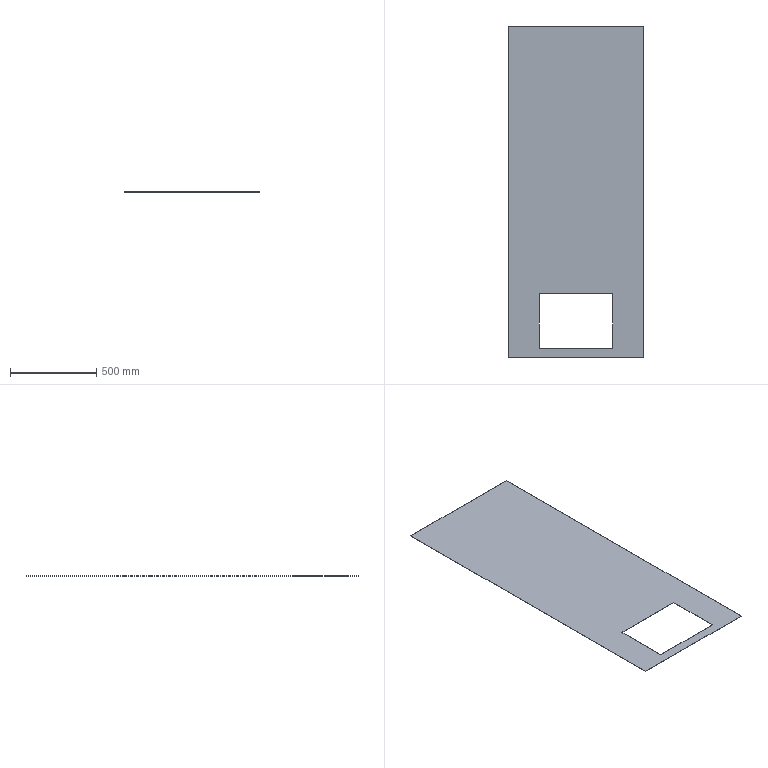Part | STEP file | 750078414 | 1 solid | 10 faces | box 785 x 1925 x 1.5 mm | volume 2064757 mm3 | plane 10
STEP:
#1=CARTESIAN_POINT('',(212.,-589.,1.5));
#2=VERTEX_POINT('',#1);
#3=CARTESIAN_POINT('',(212.,-906.5,1.5));
#4=VERTEX_POINT('',#3);
#5=CARTESIAN_POINT('',(212.,0.,1.5));
#6=DIRECTION('',(0.,-1.,0.));
#7=VECTOR('',#6,1000.);
#8=LINE('',#5,#7);
#9=EDGE_CURVE('',#2,#4,#8,.T.);
#10=ORIENTED_EDGE('',*,*,#9,.T.);
#11=CARTESIAN_POINT('',(-212.,-906.5,1.5));
#12=VERTEX_POINT('',#11);
#13=CARTESIAN_POINT('',(0.,-906.5,1.5));
#14=DIRECTION('',(-1.,0.,0.));
#15=VECTOR('',#14,1000.);
#16=LINE('',#13,#15);
#17=EDGE_CURVE('',#4,#12,#16,.T.);
#18=ORIENTED_EDGE('',*,*,#17,.T.);
#19=CARTESIAN_POINT('',(-212.,-589.,1.5));
#20=VERTEX_POINT('',#19);
#21=CARTESIAN_POINT('',(-212.,0.,1.5));
#22=DIRECTION('',(0.,1.,0.));
#23=VECTOR('',#22,1000.);
#24=LINE('',#21,#23);
#25=EDGE_CURVE('',#12,#20,#24,.T.);
#26=ORIENTED_EDGE('',*,*,#25,.T.);
#27=CARTESIAN_POINT('',(0.,-589.,1.5));
#28=DIRECTION('',(1.,0.,0.));
#29=VECTOR('',#28,1000.);
#30=LINE('',#27,#29);
#31=EDGE_CURVE('',#20,#2,#30,.T.);
#32=ORIENTED_EDGE('',*,*,#31,.T.);
#33=EDGE_LOOP('',(#10,#18,#26,#32));
#34=FACE_BOUND('',#33,.T.);
#35=CARTESIAN_POINT('',(-392.5,-962.5,1.5));
#36=VERTEX_POINT('',#35);
#37=CARTESIAN_POINT('',(392.5,-962.5,1.5));
#38=VERTEX_POINT('',#37);
#39=CARTESIAN_POINT('',(0.,-962.5,1.5));
#40=DIRECTION('',(1.,0.,0.));
#41=VECTOR('',#40,1000.);
#42=LINE('',#39,#41);
#43=EDGE_CURVE('',#36,#38,#42,.T.);
#44=ORIENTED_EDGE('',*,*,#43,.T.);
#45=CARTESIAN_POINT('',(392.5,962.5,1.5));
#46=VERTEX_POINT('',#45);
#47=CARTESIAN_POINT('',(392.5,0.,1.5));
#48=DIRECTION('',(0.,1.,0.));
#49=VECTOR('',#48,1000.);
#50=LINE('',#47,#49);
#51=EDGE_CURVE('',#38,#46,#50,.T.);
#52=ORIENTED_EDGE('',*,*,#51,.T.);
#53=CARTESIAN_POINT('',(-392.5,962.5,1.5));
#54=VERTEX_POINT('',#53);
#55=CARTESIAN_POINT('',(0.,962.5,1.5));
#56=DIRECTION('',(-1.,0.,0.));
#57=VECTOR('',#56,1000.);
#58=LINE('',#55,#57);
#59=EDGE_CURVE('',#46,#54,#58,.T.);
#60=ORIENTED_EDGE('',*,*,#59,.T.);
#61=CARTESIAN_POINT('',(-392.5,0.,1.5));
#62=DIRECTION('',(0.,-1.,0.));
#63=VECTOR('',#62,1000.);
#64=LINE('',#61,#63);
#65=EDGE_CURVE('',#54,#36,#64,.T.);
#66=ORIENTED_EDGE('',*,*,#65,.T.);
#67=EDGE_LOOP('',(#44,#52,#60,#66));
#68=FACE_OUTER_BOUND('',#67,.T.);
#69=CARTESIAN_POINT('',(0.,0.,1.5));
#70=DIRECTION('',(0.,0.,1.));
#71=DIRECTION('',(1.,0.,0.));
#72=AXIS2_PLACEMENT_3D('',#69,#70,#71);
#73=PLANE('',#72);
#74=ADVANCED_FACE('',(#34,#68),#73,.T.);
#75=CARTESIAN_POINT('',(-212.,-906.5,0.));
#76=VERTEX_POINT('',#75);
#77=CARTESIAN_POINT('',(-212.,-906.5,2078.907));
#78=DIRECTION('',(0.,0.,1.));
#79=VECTOR('',#78,1000.);
#80=LINE('',#77,#79);
#81=EDGE_CURVE('',#76,#12,#80,.T.);
#82=ORIENTED_EDGE('',*,*,#81,.T.);
#83=ORIENTED_EDGE('',*,*,#17,.F.);
#84=CARTESIAN_POINT('',(212.,-906.5,0.));
#85=VERTEX_POINT('',#84);
#86=CARTESIAN_POINT('',(212.,-906.5,2078.907));
#87=DIRECTION('',(0.,0.,-1.));
#88=VECTOR('',#87,1000.);
#89=LINE('',#86,#88);
#90=EDGE_CURVE('',#4,#85,#89,.T.);
#91=ORIENTED_EDGE('',*,*,#90,.T.);
#92=CARTESIAN_POINT('',(-212.,-906.5,0.));
#93=DIRECTION('',(-1.,0.,0.));
#94=VECTOR('',#93,1000.);
#95=LINE('',#92,#94);
#96=EDGE_CURVE('',#85,#76,#95,.T.);
#97=ORIENTED_EDGE('',*,*,#96,.T.);
#98=EDGE_LOOP('',(#82,#83,#91,#97));
#99=FACE_OUTER_BOUND('',#98,.T.);
#100=CARTESIAN_POINT('',(-212.,-906.5,2078.907));
#101=DIRECTION('',(0.,1.,0.));
#102=DIRECTION('',(0.,0.,1.));
#103=AXIS2_PLACEMENT_3D('',#100,#101,#102);
#104=PLANE('',#103);
#105=ADVANCED_FACE('',(#99),#104,.T.);
#106=ORIENTED_EDGE('',*,*,#90,.F.);
#107=ORIENTED_EDGE('',*,*,#9,.F.);
#108=CARTESIAN_POINT('',(212.,-589.,0.));
#109=VERTEX_POINT('',#108);
#110=CARTESIAN_POINT('',(212.,-589.,2078.907));
#111=DIRECTION('',(0.,0.,-1.));
#112=VECTOR('',#111,1000.);
#113=LINE('',#110,#112);
#114=EDGE_CURVE('',#2,#109,#113,.T.);
#115=ORIENTED_EDGE('',*,*,#114,.T.);
#116=CARTESIAN_POINT('',(212.,-906.5,0.));
#117=DIRECTION('',(0.,-1.,0.));
#118=VECTOR('',#117,1000.);
#119=LINE('',#116,#118);
#120=EDGE_CURVE('',#109,#85,#119,.T.);
#121=ORIENTED_EDGE('',*,*,#120,.T.);
#122=EDGE_LOOP('',(#106,#107,#115,#121));
#123=FACE_OUTER_BOUND('',#122,.T.);
#124=CARTESIAN_POINT('',(212.,-906.5,2078.907));
#125=DIRECTION('',(-1.,0.,0.));
#126=DIRECTION('',(0.,-1.,0.));
#127=AXIS2_PLACEMENT_3D('',#124,#125,#126);
#128=PLANE('',#127);
#129=ADVANCED_FACE('',(#123),#128,.T.);
#130=ORIENTED_EDGE('',*,*,#114,.F.);
#131=ORIENTED_EDGE('',*,*,#31,.F.);
#132=CARTESIAN_POINT('',(-212.,-589.,0.));
#133=VERTEX_POINT('',#132);
#134=CARTESIAN_POINT('',(-212.,-589.,2078.907));
#135=DIRECTION('',(0.,0.,-1.));
#136=VECTOR('',#135,1000.);
#137=LINE('',#134,#136);
#138=EDGE_CURVE('',#20,#133,#137,.T.);
#139=ORIENTED_EDGE('',*,*,#138,.T.);
#140=CARTESIAN_POINT('',(212.,-589.,0.));
#141=DIRECTION('',(1.,0.,0.));
#142=VECTOR('',#141,1000.);
#143=LINE('',#140,#142);
#144=EDGE_CURVE('',#133,#109,#143,.T.);
#145=ORIENTED_EDGE('',*,*,#144,.T.);
#146=EDGE_LOOP('',(#130,#131,#139,#145));
#147=FACE_OUTER_BOUND('',#146,.T.);
#148=CARTESIAN_POINT('',(212.,-589.,2078.907));
#149=DIRECTION('',(0.,-1.,0.));
#150=DIRECTION('',(0.,0.,-1.));
#151=AXIS2_PLACEMENT_3D('',#148,#149,#150);
#152=PLANE('',#151);
#153=ADVANCED_FACE('',(#147),#152,.T.);
#154=ORIENTED_EDGE('',*,*,#138,.F.);
#155=ORIENTED_EDGE('',*,*,#25,.F.);
#156=ORIENTED_EDGE('',*,*,#81,.F.);
#157=CARTESIAN_POINT('',(-212.,-589.,0.));
#158=DIRECTION('',(0.,1.,0.));
#159=VECTOR('',#158,1000.);
#160=LINE('',#157,#159);
#161=EDGE_CURVE('',#76,#133,#160,.T.);
#162=ORIENTED_EDGE('',*,*,#161,.T.);
#163=EDGE_LOOP('',(#154,#155,#156,#162));
#164=FACE_OUTER_BOUND('',#163,.T.);
#165=CARTESIAN_POINT('',(-212.,-589.,2078.907));
#166=DIRECTION('',(1.,0.,0.));
#167=DIRECTION('',(0.,1.,0.));
#168=AXIS2_PLACEMENT_3D('',#165,#166,#167);
#169=PLANE('',#168);
#170=ADVANCED_FACE('',(#164),#169,.T.);
#171=CARTESIAN_POINT('',(392.5,962.5,0.));
#172=VERTEX_POINT('',#171);
#173=CARTESIAN_POINT('',(392.5,962.5,1.5));
#174=DIRECTION('',(0.,0.,-1.));
#175=VECTOR('',#174,1000.);
#176=LINE('',#173,#175);
#177=EDGE_CURVE('',#46,#172,#176,.T.);
#178=ORIENTED_EDGE('',*,*,#177,.F.);
#179=ORIENTED_EDGE('',*,*,#51,.F.);
#180=CARTESIAN_POINT('',(392.5,-962.5,0.));
#181=VERTEX_POINT('',#180);
#182=CARTESIAN_POINT('',(392.5,-962.5,1.5));
#183=DIRECTION('',(0.,0.,1.));
#184=VECTOR('',#183,1000.);
#185=LINE('',#182,#184);
#186=EDGE_CURVE('',#181,#38,#185,.T.);
#187=ORIENTED_EDGE('',*,*,#186,.F.);
#188=CARTESIAN_POINT('',(392.5,-962.5,0.));
#189=DIRECTION('',(0.,-1.,0.));
#190=VECTOR('',#189,1000.);
#191=LINE('',#188,#190);
#192=EDGE_CURVE('',#172,#181,#191,.T.);
#193=ORIENTED_EDGE('',*,*,#192,.F.);
#194=EDGE_LOOP('',(#178,#179,#187,#193));
#195=FACE_OUTER_BOUND('',#194,.T.);
#196=CARTESIAN_POINT('',(392.5,-962.5,1.5));
#197=DIRECTION('',(-1.,0.,0.));
#198=DIRECTION('',(0.,0.,1.));
#199=AXIS2_PLACEMENT_3D('',#196,#197,#198);
#200=PLANE('',#199);
#201=ADVANCED_FACE('',(#195),#200,.F.);
#202=ORIENTED_EDGE('',*,*,#186,.T.);
#203=ORIENTED_EDGE('',*,*,#43,.F.);
#204=CARTESIAN_POINT('',(-392.5,-962.5,0.));
#205=VERTEX_POINT('',#204);
#206=CARTESIAN_POINT('',(-392.5,-962.5,1.5));
#207=DIRECTION('',(0.,0.,1.));
#208=VECTOR('',#207,1000.);
#209=LINE('',#206,#208);
#210=EDGE_CURVE('',#205,#36,#209,.T.);
#211=ORIENTED_EDGE('',*,*,#210,.F.);
#212=CARTESIAN_POINT('',(-392.5,-962.5,0.));
#213=DIRECTION('',(-1.,0.,0.));
#214=VECTOR('',#213,1000.);
#215=LINE('',#212,#214);
#216=EDGE_CURVE('',#181,#205,#215,.T.);
#217=ORIENTED_EDGE('',*,*,#216,.F.);
#218=EDGE_LOOP('',(#202,#203,#211,#217));
#219=FACE_OUTER_BOUND('',#218,.T.);
#220=CARTESIAN_POINT('',(-392.5,-962.5,1.5));
#221=DIRECTION('',(0.,1.,0.));
#222=DIRECTION('',(0.,0.,1.));
#223=AXIS2_PLACEMENT_3D('',#220,#221,#222);
#224=PLANE('',#223);
#225=ADVANCED_FACE('',(#219),#224,.F.);
#226=ORIENTED_EDGE('',*,*,#210,.T.);
#227=ORIENTED_EDGE('',*,*,#65,.F.);
#228=CARTESIAN_POINT('',(-392.5,962.5,0.));
#229=VERTEX_POINT('',#228);
#230=CARTESIAN_POINT('',(-392.5,962.5,1.5));
#231=DIRECTION('',(0.,0.,1.));
#232=VECTOR('',#231,1000.);
#233=LINE('',#230,#232);
#234=EDGE_CURVE('',#229,#54,#233,.T.);
#235=ORIENTED_EDGE('',*,*,#234,.F.);
#236=CARTESIAN_POINT('',(-392.5,962.5,0.));
#237=DIRECTION('',(0.,1.,0.));
#238=VECTOR('',#237,1000.);
#239=LINE('',#236,#238);
#240=EDGE_CURVE('',#205,#229,#239,.T.);
#241=ORIENTED_EDGE('',*,*,#240,.F.);
#242=EDGE_LOOP('',(#226,#227,#235,#241));
#243=FACE_OUTER_BOUND('',#242,.T.);
#244=CARTESIAN_POINT('',(-392.5,962.5,1.5));
#245=DIRECTION('',(1.,0.,0.));
#246=DIRECTION('',(0.,0.,-1.));
#247=AXIS2_PLACEMENT_3D('',#244,#245,#246);
#248=PLANE('',#247);
#249=ADVANCED_FACE('',(#243),#248,.F.);
#250=ORIENTED_EDGE('',*,*,#234,.T.);
#251=ORIENTED_EDGE('',*,*,#59,.F.);
#252=ORIENTED_EDGE('',*,*,#177,.T.);
#253=CARTESIAN_POINT('',(392.5,962.5,0.));
#254=DIRECTION('',(1.,0.,0.));
#255=VECTOR('',#254,1000.);
#256=LINE('',#253,#255);
#257=EDGE_CURVE('',#229,#172,#256,.T.);
#258=ORIENTED_EDGE('',*,*,#257,.F.);
#259=EDGE_LOOP('',(#250,#251,#252,#258));
#260=FACE_OUTER_BOUND('',#259,.T.);
#261=CARTESIAN_POINT('',(392.5,962.5,1.5));
#262=DIRECTION('',(0.,-1.,0.));
#263=DIRECTION('',(0.,0.,-1.));
#264=AXIS2_PLACEMENT_3D('',#261,#262,#263);
#265=PLANE('',#264);
#266=ADVANCED_FACE('',(#260),#265,.F.);
#267=ORIENTED_EDGE('',*,*,#161,.F.);
#268=ORIENTED_EDGE('',*,*,#96,.F.);
#269=ORIENTED_EDGE('',*,*,#120,.F.);
#270=ORIENTED_EDGE('',*,*,#144,.F.);
#271=EDGE_LOOP('',(#267,#268,#269,#270));
#272=FACE_BOUND('',#271,.T.);
#273=ORIENTED_EDGE('',*,*,#192,.T.);
#274=ORIENTED_EDGE('',*,*,#216,.T.);
#275=ORIENTED_EDGE('',*,*,#240,.T.);
#276=ORIENTED_EDGE('',*,*,#257,.T.);
#277=EDGE_LOOP('',(#273,#274,#275,#276));
#278=FACE_OUTER_BOUND('',#277,.T.);
#279=CARTESIAN_POINT('',(0.,0.,0.));
#280=DIRECTION('',(0.,0.,1.));
#281=DIRECTION('',(1.,0.,0.));
#282=AXIS2_PLACEMENT_3D('',#279,#280,#281);
#283=PLANE('',#282);
#284=ADVANCED_FACE('',(#272,#278),#283,.F.);
#285=CLOSED_SHELL('',(#74,#105,#129,#153,#170,#201,#225,#249,#266,#284));
#286=MANIFOLD_SOLID_BREP('',#285);
#287=CARTESIAN_POINT('',(0.,0.,0.));
#288=DIRECTION('',(0.,0.,1.));
#289=DIRECTION('',(1.,0.,0.));
#290=AXIS2_PLACEMENT_3D('',#287,#288,#289);
#291=(LENGTH_UNIT()NAMED_UNIT(*)SI_UNIT(.MILLI.,.METRE.));
#292=UNCERTAINTY_MEASURE_WITH_UNIT(LENGTH_MEASURE(0.00001),#291,'','');
#293=(NAMED_UNIT(*)PLANE_ANGLE_UNIT()SI_UNIT($,.RADIAN.));
#294=(NAMED_UNIT(*)SI_UNIT($,.STERADIAN.)SOLID_ANGLE_UNIT());
#295=(GEOMETRIC_REPRESENTATION_CONTEXT(3)GLOBAL_UNCERTAINTY_ASSIGNED_CONTEXT((#292))GLOBAL_UNIT_ASSIGNED_CONTEXT((#291,#293,#294))REPRESENTATION_CONTEXT('',''));
#296=ADVANCED_BREP_SHAPE_REPRESENTATION('',(#286,#290),#295);